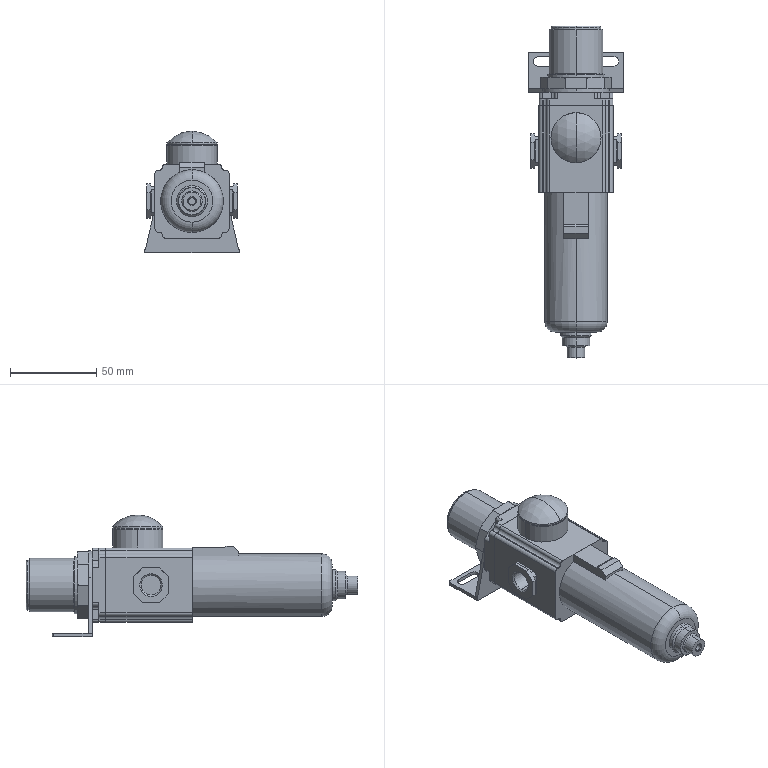Part | SolidWorks | features BaseBody 1 | 1 solid | 223 faces | box 55 x 192.5 x 70.622 mm | volume 237290 mm3 | plane 119 | cylinder 72 | torus 16 | cone 14 | sphere 2 | commonest cylinder face diameters 4 x24 3 x12 5.4 x6 29 x6 11.445 x4 2 x2